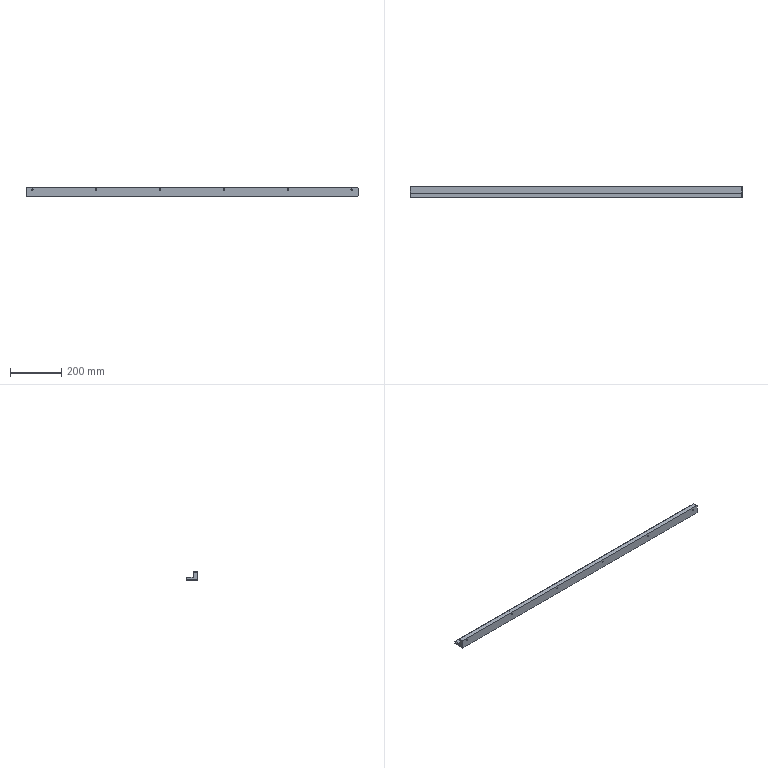Part | NX | features BREP 1 | 1 solid | 68 faces | box 1300 x 44 x 35 mm | volume 1189341 mm3 | cylinder 36 | plane 20 | cone 12 | commonest cylinder face diameters 3.3 x12 5.5 x12 10 x12